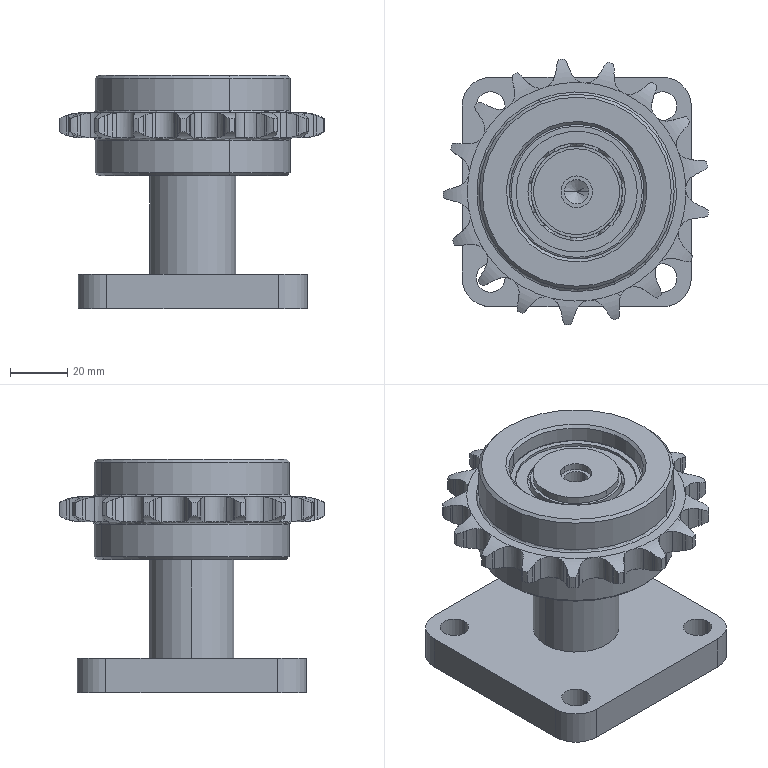Part | NX | features BREP 5 | 6 solids | 675 faces | box 92.535 x 92.741 x 81.5 mm | volume 212847 mm3 | sphere 240 | cylinder 192 | torus 122 | plane 107 | cone 14 | commonest cylinder face diameters 14.871 x36 26.567 x35 10.311 x22 93 x17 42.3 x16 25 x10